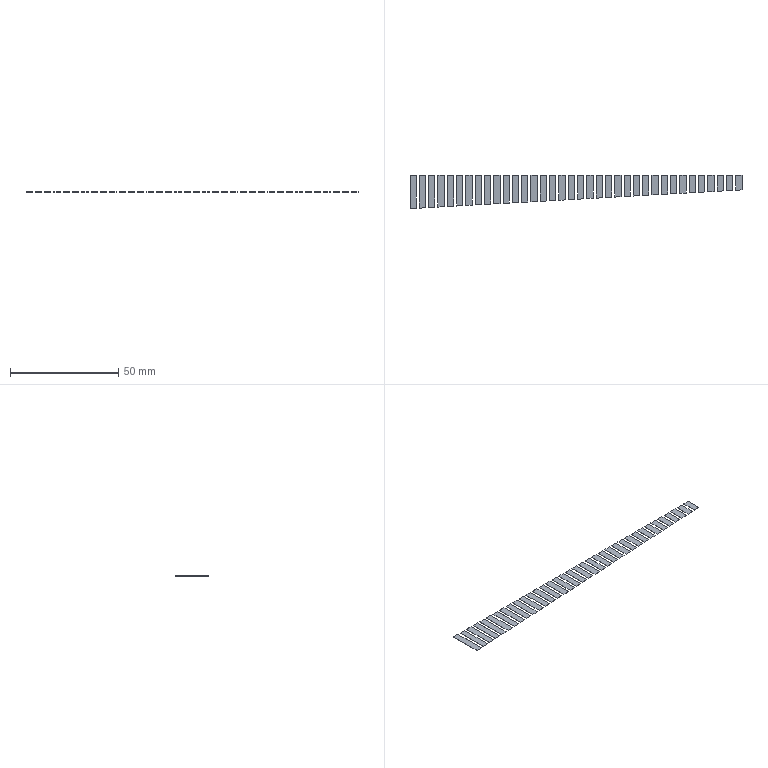Part | SolidWorks | features Extrusion 1, ICE 1 | 36 solids | 216 faces | box 153.4 x 15.412 x 0.1 mm | volume 115.568 mm3 | plane 216